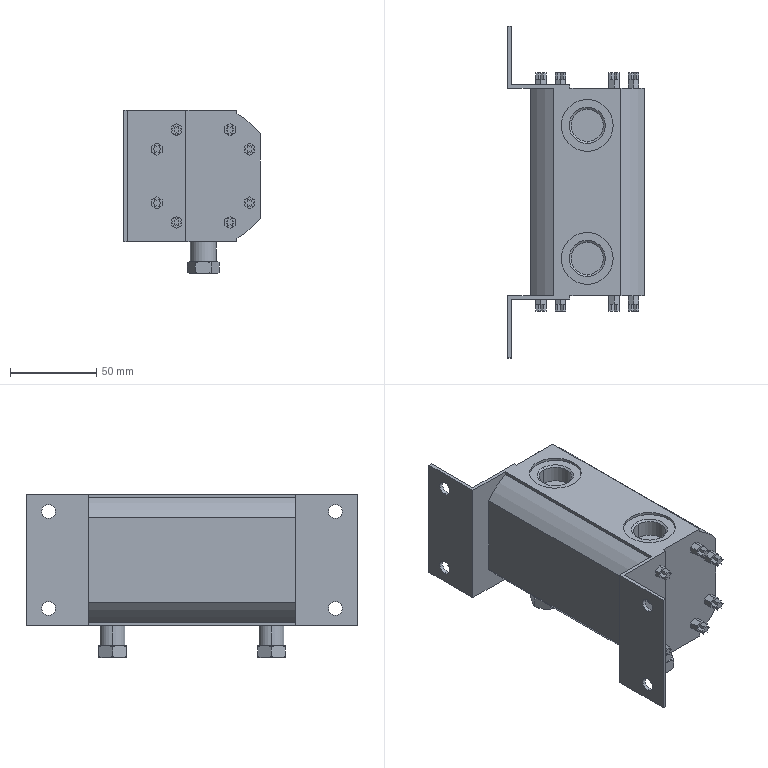Part | STEP file | 4-20.sldasm-Part-129 | 1 solid | 502 faces | box 79 x 192 x 94.5 mm | volume 576073 mm3 | plane 444 | cone 30 | cylinder 28 | commonest cylinder face diameters 8 x8 18.631 x6 30 x6 15 x4 82 x4